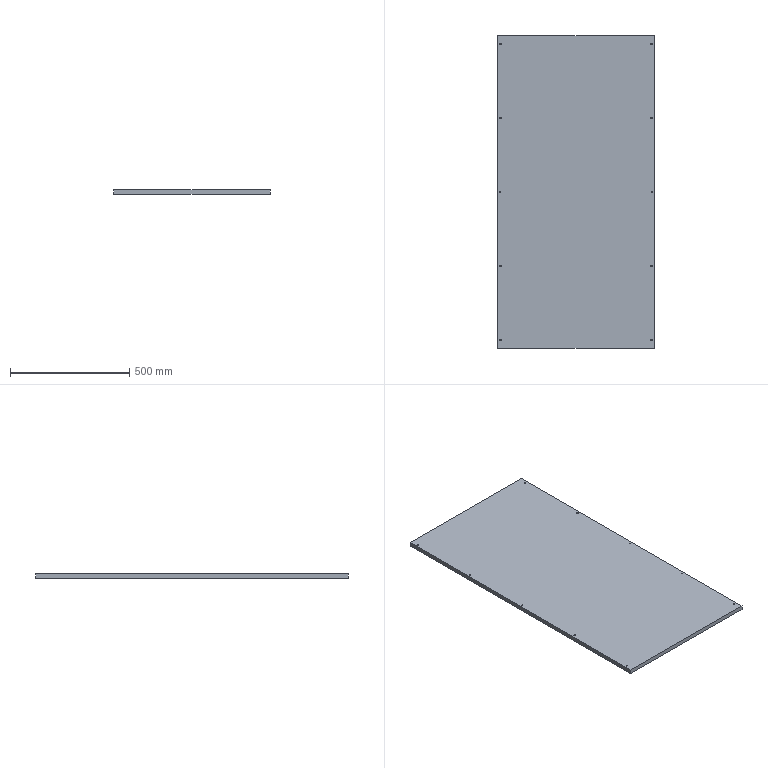Part | STEP file | DECAK NQ7A | 1 solid | 16 faces | box 658 x 1310 x 18 mm | volume 15510409 mm3 | cylinder 10 | plane 6 | commonest cylinder face diameters 6.5 x8 4 x2
STEP:
#1=CARTESIAN_POINT('',(0.,0.,0.));
#2=DIRECTION('',(0.,0.,1.));
#3=DIRECTION('',(1.,0.,0.));
#4=AXIS2_PLACEMENT_3D('',#1,#2,#3);
#5=CARTESIAN_POINT('',(320.75,-620.,9.));
#6=VERTEX_POINT('',#5);
#7=CARTESIAN_POINT('',(317.5,-620.,9.));
#8=DIRECTION('',(0.,0.,1.));
#9=DIRECTION('',(1.,0.,0.));
#10=AXIS2_PLACEMENT_3D('',#7,#8,#9);
#11=CIRCLE('',#10,3.25);
#12=CARTESIAN_POINT('',(329.,-655.,9.));
#13=DIRECTION('',(0.,0.,1.));
#14=DIRECTION('',(1.,0.,0.));
#15=AXIS2_PLACEMENT_3D('',#12,#13,#14);
#16=PLANE('',#15);
#17=CARTESIAN_POINT('',(-11.5,35.));
#18=DIRECTION('',(1.,0.));
#19=AXIS2_PLACEMENT_2D('',#17,#18);
#20=CIRCLE('',#19,3.25);
#21=(GEOMETRIC_REPRESENTATION_CONTEXT(2)PARAMETRIC_REPRESENTATION_CONTEXT()REPRESENTATION_CONTEXT('',''));
#22=DEFINITIONAL_REPRESENTATION('',(#20),#21);
#23=PCURVE('',#16,#22);
#24=CARTESIAN_POINT('',(317.5,-620.,9.));
#25=DIRECTION('',(0.,0.,-1.));
#26=DIRECTION('',(-1.,0.,0.));
#27=AXIS2_PLACEMENT_3D('',#24,#25,#26);
#28=CYLINDRICAL_SURFACE('',#27,3.25);
#29=CARTESIAN_POINT('',(9.425,0.));
#30=DIRECTION('',(-1.,0.));
#31=VECTOR('',#30,1.);
#32=LINE('',#29,#31);
#33=(GEOMETRIC_REPRESENTATION_CONTEXT(2)PARAMETRIC_REPRESENTATION_CONTEXT()REPRESENTATION_CONTEXT('',''));
#34=DEFINITIONAL_REPRESENTATION('',(#32),#33);
#35=PCURVE('',#28,#34);
#36=SURFACE_CURVE('',#11,(#23,#35),.PCURVE_S1.);
#37=EDGE_CURVE('',#6,#6,#36,.T.);
#38=ORIENTED_EDGE('',*,*,#37,.F.);
#39=EDGE_LOOP('',(#38));
#40=FACE_BOUND('',#39,.T.);
#41=CARTESIAN_POINT('',(320.75,-310.,9.));
#42=VERTEX_POINT('',#41);
#43=CARTESIAN_POINT('',(317.5,-310.,9.));
#44=DIRECTION('',(0.,0.,1.));
#45=DIRECTION('',(1.,0.,0.));
#46=AXIS2_PLACEMENT_3D('',#43,#44,#45);
#47=CIRCLE('',#46,3.25);
#48=CARTESIAN_POINT('',(-11.5,345.));
#49=DIRECTION('',(1.,0.));
#50=AXIS2_PLACEMENT_2D('',#48,#49);
#51=CIRCLE('',#50,3.25);
#52=(GEOMETRIC_REPRESENTATION_CONTEXT(2)PARAMETRIC_REPRESENTATION_CONTEXT()REPRESENTATION_CONTEXT('',''));
#53=DEFINITIONAL_REPRESENTATION('',(#51),#52);
#54=PCURVE('',#16,#53);
#55=CARTESIAN_POINT('',(317.5,-310.,9.));
#56=DIRECTION('',(0.,0.,-1.));
#57=DIRECTION('',(-1.,0.,0.));
#58=AXIS2_PLACEMENT_3D('',#55,#56,#57);
#59=CYLINDRICAL_SURFACE('',#58,3.25);
#60=CARTESIAN_POINT('',(9.425,0.));
#61=DIRECTION('',(-1.,0.));
#62=VECTOR('',#61,1.);
#63=LINE('',#60,#62);
#64=(GEOMETRIC_REPRESENTATION_CONTEXT(2)PARAMETRIC_REPRESENTATION_CONTEXT()REPRESENTATION_CONTEXT('',''));
#65=DEFINITIONAL_REPRESENTATION('',(#63),#64);
#66=PCURVE('',#59,#65);
#67=SURFACE_CURVE('',#47,(#54,#66),.PCURVE_S1.);
#68=EDGE_CURVE('',#42,#42,#67,.T.);
#69=ORIENTED_EDGE('',*,*,#68,.F.);
#70=EDGE_LOOP('',(#69));
#71=FACE_BOUND('',#70,.T.);
#72=CARTESIAN_POINT('',(319.5,0.,9.));
#73=VERTEX_POINT('',#72);
#74=CARTESIAN_POINT('',(317.5,0.,9.));
#75=DIRECTION('',(0.,0.,1.));
#76=DIRECTION('',(1.,0.,0.));
#77=AXIS2_PLACEMENT_3D('',#74,#75,#76);
#78=CIRCLE('',#77,2.);
#79=CARTESIAN_POINT('',(-11.5,655.));
#80=DIRECTION('',(1.,0.));
#81=AXIS2_PLACEMENT_2D('',#79,#80);
#82=CIRCLE('',#81,2.);
#83=(GEOMETRIC_REPRESENTATION_CONTEXT(2)PARAMETRIC_REPRESENTATION_CONTEXT()REPRESENTATION_CONTEXT('',''));
#84=DEFINITIONAL_REPRESENTATION('',(#82),#83);
#85=PCURVE('',#16,#84);
#86=CARTESIAN_POINT('',(317.5,0.,9.));
#87=DIRECTION('',(0.,0.,-1.));
#88=DIRECTION('',(-1.,0.,0.));
#89=AXIS2_PLACEMENT_3D('',#86,#87,#88);
#90=CYLINDRICAL_SURFACE('',#89,2.);
#91=CARTESIAN_POINT('',(9.425,0.));
#92=DIRECTION('',(-1.,0.));
#93=VECTOR('',#92,1.);
#94=LINE('',#91,#93);
#95=(GEOMETRIC_REPRESENTATION_CONTEXT(2)PARAMETRIC_REPRESENTATION_CONTEXT()REPRESENTATION_CONTEXT('',''));
#96=DEFINITIONAL_REPRESENTATION('',(#94),#95);
#97=PCURVE('',#90,#96);
#98=SURFACE_CURVE('',#78,(#85,#97),.PCURVE_S1.);
#99=EDGE_CURVE('',#73,#73,#98,.T.);
#100=ORIENTED_EDGE('',*,*,#99,.F.);
#101=EDGE_LOOP('',(#100));
#102=FACE_BOUND('',#101,.T.);
#103=CARTESIAN_POINT('',(-314.25,310.,9.));
#104=VERTEX_POINT('',#103);
#105=CARTESIAN_POINT('',(-317.5,310.,9.));
#106=DIRECTION('',(0.,0.,1.));
#107=DIRECTION('',(1.,0.,0.));
#108=AXIS2_PLACEMENT_3D('',#105,#106,#107);
#109=CIRCLE('',#108,3.25);
#110=CARTESIAN_POINT('',(-646.5,965.));
#111=DIRECTION('',(1.,0.));
#112=AXIS2_PLACEMENT_2D('',#110,#111);
#113=CIRCLE('',#112,3.25);
#114=(GEOMETRIC_REPRESENTATION_CONTEXT(2)PARAMETRIC_REPRESENTATION_CONTEXT()REPRESENTATION_CONTEXT('',''));
#115=DEFINITIONAL_REPRESENTATION('',(#113),#114);
#116=PCURVE('',#16,#115);
#117=CARTESIAN_POINT('',(-317.5,310.,9.));
#118=DIRECTION('',(0.,0.,-1.));
#119=DIRECTION('',(-1.,0.,0.));
#120=AXIS2_PLACEMENT_3D('',#117,#118,#119);
#121=CYLINDRICAL_SURFACE('',#120,3.25);
#122=CARTESIAN_POINT('',(9.425,0.));
#123=DIRECTION('',(-1.,0.));
#124=VECTOR('',#123,1.);
#125=LINE('',#122,#124);
#126=(GEOMETRIC_REPRESENTATION_CONTEXT(2)PARAMETRIC_REPRESENTATION_CONTEXT()REPRESENTATION_CONTEXT('',''));
#127=DEFINITIONAL_REPRESENTATION('',(#125),#126);
#128=PCURVE('',#121,#127);
#129=SURFACE_CURVE('',#109,(#116,#128),.PCURVE_S1.);
#130=EDGE_CURVE('',#104,#104,#129,.T.);
#131=ORIENTED_EDGE('',*,*,#130,.F.);
#132=EDGE_LOOP('',(#131));
#133=FACE_BOUND('',#132,.T.);
#134=CARTESIAN_POINT('',(320.75,620.,9.));
#135=VERTEX_POINT('',#134);
#136=CARTESIAN_POINT('',(317.5,620.,9.));
#137=DIRECTION('',(0.,0.,1.));
#138=DIRECTION('',(1.,0.,0.));
#139=AXIS2_PLACEMENT_3D('',#136,#137,#138);
#140=CIRCLE('',#139,3.25);
#141=CARTESIAN_POINT('',(-11.5,1275.));
#142=DIRECTION('',(1.,0.));
#143=AXIS2_PLACEMENT_2D('',#141,#142);
#144=CIRCLE('',#143,3.25);
#145=(GEOMETRIC_REPRESENTATION_CONTEXT(2)PARAMETRIC_REPRESENTATION_CONTEXT()REPRESENTATION_CONTEXT('',''));
#146=DEFINITIONAL_REPRESENTATION('',(#144),#145);
#147=PCURVE('',#16,#146);
#148=CARTESIAN_POINT('',(317.5,620.,9.));
#149=DIRECTION('',(0.,0.,-1.));
#150=DIRECTION('',(-1.,0.,0.));
#151=AXIS2_PLACEMENT_3D('',#148,#149,#150);
#152=CYLINDRICAL_SURFACE('',#151,3.25);
#153=CARTESIAN_POINT('',(9.425,0.));
#154=DIRECTION('',(-1.,0.));
#155=VECTOR('',#154,1.);
#156=LINE('',#153,#155);
#157=(GEOMETRIC_REPRESENTATION_CONTEXT(2)PARAMETRIC_REPRESENTATION_CONTEXT()REPRESENTATION_CONTEXT('',''));
#158=DEFINITIONAL_REPRESENTATION('',(#156),#157);
#159=PCURVE('',#152,#158);
#160=SURFACE_CURVE('',#140,(#147,#159),.PCURVE_S1.);
#161=EDGE_CURVE('',#135,#135,#160,.T.);
#162=ORIENTED_EDGE('',*,*,#161,.F.);
#163=EDGE_LOOP('',(#162));
#164=FACE_BOUND('',#163,.T.);
#165=CARTESIAN_POINT('',(329.,-655.,9.));
#166=VERTEX_POINT('',#165);
#167=CARTESIAN_POINT('',(329.,655.,9.));
#168=VERTEX_POINT('',#167);
#169=CARTESIAN_POINT('',(329.,655.,9.));
#170=DIRECTION('',(0.,1.,0.));
#171=VECTOR('',#170,1.);
#172=LINE('',#169,#171);
#173=CARTESIAN_POINT('',(0.,1310.));
#174=DIRECTION('',(0.,1.));
#175=VECTOR('',#174,1.);
#176=LINE('',#173,#175);
#177=(GEOMETRIC_REPRESENTATION_CONTEXT(2)PARAMETRIC_REPRESENTATION_CONTEXT()REPRESENTATION_CONTEXT('',''));
#178=DEFINITIONAL_REPRESENTATION('',(#176),#177);
#179=PCURVE('',#16,#178);
#180=CARTESIAN_POINT('',(329.,655.,9.));
#181=DIRECTION('',(-1.,0.,0.));
#182=DIRECTION('',(0.,0.,1.));
#183=AXIS2_PLACEMENT_3D('',#180,#181,#182);
#184=PLANE('',#183);
#185=CARTESIAN_POINT('',(0.,0.));
#186=DIRECTION('',(0.,1.));
#187=VECTOR('',#186,1.);
#188=LINE('',#185,#187);
#189=(GEOMETRIC_REPRESENTATION_CONTEXT(2)PARAMETRIC_REPRESENTATION_CONTEXT()REPRESENTATION_CONTEXT('',''));
#190=DEFINITIONAL_REPRESENTATION('',(#188),#189);
#191=PCURVE('',#184,#190);
#192=SURFACE_CURVE('',#172,(#179,#191),.PCURVE_S1.);
#193=EDGE_CURVE('',#166,#168,#192,.T.);
#194=ORIENTED_EDGE('',*,*,#193,.T.);
#195=CARTESIAN_POINT('',(-329.,655.,9.));
#196=VERTEX_POINT('',#195);
#197=CARTESIAN_POINT('',(-329.,655.,9.));
#198=DIRECTION('',(-1.,0.,0.));
#199=VECTOR('',#198,1.);
#200=LINE('',#197,#199);
#201=CARTESIAN_POINT('',(-658.,1310.));
#202=DIRECTION('',(-1.,0.));
#203=VECTOR('',#202,1.);
#204=LINE('',#201,#203);
#205=(GEOMETRIC_REPRESENTATION_CONTEXT(2)PARAMETRIC_REPRESENTATION_CONTEXT()REPRESENTATION_CONTEXT('',''));
#206=DEFINITIONAL_REPRESENTATION('',(#204),#205);
#207=PCURVE('',#16,#206);
#208=CARTESIAN_POINT('',(-329.,655.,9.));
#209=DIRECTION('',(0.,-1.,0.));
#210=DIRECTION('',(1.,0.,0.));
#211=AXIS2_PLACEMENT_3D('',#208,#209,#210);
#212=PLANE('',#211);
#213=CARTESIAN_POINT('',(0.,0.));
#214=DIRECTION('',(-1.,0.));
#215=VECTOR('',#214,1.);
#216=LINE('',#213,#215);
#217=(GEOMETRIC_REPRESENTATION_CONTEXT(2)PARAMETRIC_REPRESENTATION_CONTEXT()REPRESENTATION_CONTEXT('',''));
#218=DEFINITIONAL_REPRESENTATION('',(#216),#217);
#219=PCURVE('',#212,#218);
#220=SURFACE_CURVE('',#200,(#207,#219),.PCURVE_S1.);
#221=EDGE_CURVE('',#168,#196,#220,.T.);
#222=ORIENTED_EDGE('',*,*,#221,.T.);
#223=CARTESIAN_POINT('',(-329.,-655.,9.));
#224=VERTEX_POINT('',#223);
#225=CARTESIAN_POINT('',(-329.,655.,9.));
#226=DIRECTION('',(0.,-1.,0.));
#227=VECTOR('',#226,1.);
#228=LINE('',#225,#227);
#229=CARTESIAN_POINT('',(-658.,1310.));
#230=DIRECTION('',(0.,-1.));
#231=VECTOR('',#230,1.);
#232=LINE('',#229,#231);
#233=(GEOMETRIC_REPRESENTATION_CONTEXT(2)PARAMETRIC_REPRESENTATION_CONTEXT()REPRESENTATION_CONTEXT('',''));
#234=DEFINITIONAL_REPRESENTATION('',(#232),#233);
#235=PCURVE('',#16,#234);
#236=CARTESIAN_POINT('',(-329.,655.,9.));
#237=DIRECTION('',(1.,0.,0.));
#238=DIRECTION('',(0.,0.,-1.));
#239=AXIS2_PLACEMENT_3D('',#236,#237,#238);
#240=PLANE('',#239);
#241=CARTESIAN_POINT('',(0.,0.));
#242=DIRECTION('',(0.,-1.));
#243=VECTOR('',#242,1.);
#244=LINE('',#241,#243);
#245=(GEOMETRIC_REPRESENTATION_CONTEXT(2)PARAMETRIC_REPRESENTATION_CONTEXT()REPRESENTATION_CONTEXT('',''));
#246=DEFINITIONAL_REPRESENTATION('',(#244),#245);
#247=PCURVE('',#240,#246);
#248=SURFACE_CURVE('',#228,(#235,#247),.PCURVE_S1.);
#249=EDGE_CURVE('',#196,#224,#248,.T.);
#250=ORIENTED_EDGE('',*,*,#249,.T.);
#251=CARTESIAN_POINT('',(-329.,-655.,9.));
#252=DIRECTION('',(1.,0.,0.));
#253=VECTOR('',#252,1.);
#254=LINE('',#251,#253);
#255=CARTESIAN_POINT('',(-658.,0.));
#256=DIRECTION('',(1.,0.));
#257=VECTOR('',#256,1.);
#258=LINE('',#255,#257);
#259=(GEOMETRIC_REPRESENTATION_CONTEXT(2)PARAMETRIC_REPRESENTATION_CONTEXT()REPRESENTATION_CONTEXT('',''));
#260=DEFINITIONAL_REPRESENTATION('',(#258),#259);
#261=PCURVE('',#16,#260);
#262=CARTESIAN_POINT('',(-329.,-655.,9.));
#263=DIRECTION('',(0.,1.,0.));
#264=DIRECTION('',(-1.,0.,0.));
#265=AXIS2_PLACEMENT_3D('',#262,#263,#264);
#266=PLANE('',#265);
#267=CARTESIAN_POINT('',(0.,0.));
#268=DIRECTION('',(-1.,0.));
#269=VECTOR('',#268,1.);
#270=LINE('',#267,#269);
#271=(GEOMETRIC_REPRESENTATION_CONTEXT(2)PARAMETRIC_REPRESENTATION_CONTEXT()REPRESENTATION_CONTEXT('',''));
#272=DEFINITIONAL_REPRESENTATION('',(#270),#271);
#273=PCURVE('',#266,#272);
#274=SURFACE_CURVE('',#254,(#261,#273),.PCURVE_S1.);
#275=EDGE_CURVE('',#224,#166,#274,.T.);
#276=ORIENTED_EDGE('',*,*,#275,.T.);
#277=EDGE_LOOP('',(#194,#222,#250,#276));
#278=FACE_BOUND('',#277,.T.);
#279=CARTESIAN_POINT('',(-314.25,620.,9.));
#280=VERTEX_POINT('',#279);
#281=CARTESIAN_POINT('',(-317.5,620.,9.));
#282=DIRECTION('',(0.,0.,1.));
#283=DIRECTION('',(1.,0.,0.));
#284=AXIS2_PLACEMENT_3D('',#281,#282,#283);
#285=CIRCLE('',#284,3.25);
#286=CARTESIAN_POINT('',(-646.5,1275.));
#287=DIRECTION('',(1.,0.));
#288=AXIS2_PLACEMENT_2D('',#286,#287);
#289=CIRCLE('',#288,3.25);
#290=(GEOMETRIC_REPRESENTATION_CONTEXT(2)PARAMETRIC_REPRESENTATION_CONTEXT()REPRESENTATION_CONTEXT('',''));
#291=DEFINITIONAL_REPRESENTATION('',(#289),#290);
#292=PCURVE('',#16,#291);
#293=CARTESIAN_POINT('',(-317.5,620.,9.));
#294=DIRECTION('',(0.,0.,-1.));
#295=DIRECTION('',(-1.,0.,0.));
#296=AXIS2_PLACEMENT_3D('',#293,#294,#295);
#297=CYLINDRICAL_SURFACE('',#296,3.25);
#298=CARTESIAN_POINT('',(9.425,0.));
#299=DIRECTION('',(-1.,0.));
#300=VECTOR('',#299,1.);
#301=LINE('',#298,#300);
#302=(GEOMETRIC_REPRESENTATION_CONTEXT(2)PARAMETRIC_REPRESENTATION_CONTEXT()REPRESENTATION_CONTEXT('',''));
#303=DEFINITIONAL_REPRESENTATION('',(#301),#302);
#304=PCURVE('',#297,#303);
#305=SURFACE_CURVE('',#285,(#292,#304),.PCURVE_S1.);
#306=EDGE_CURVE('',#280,#280,#305,.T.);
#307=ORIENTED_EDGE('',*,*,#306,.F.);
#308=EDGE_LOOP('',(#307));
#309=FACE_BOUND('',#308,.T.);
#310=CARTESIAN_POINT('',(320.75,310.,9.));
#311=VERTEX_POINT('',#310);
#312=CARTESIAN_POINT('',(317.5,310.,9.));
#313=DIRECTION('',(0.,0.,1.));
#314=DIRECTION('',(1.,0.,0.));
#315=AXIS2_PLACEMENT_3D('',#312,#313,#314);
#316=CIRCLE('',#315,3.25);
#317=CARTESIAN_POINT('',(-11.5,965.));
#318=DIRECTION('',(1.,0.));
#319=AXIS2_PLACEMENT_2D('',#317,#318);
#320=CIRCLE('',#319,3.25);
#321=(GEOMETRIC_REPRESENTATION_CONTEXT(2)PARAMETRIC_REPRESENTATION_CONTEXT()REPRESENTATION_CONTEXT('',''));
#322=DEFINITIONAL_REPRESENTATION('',(#320),#321);
#323=PCURVE('',#16,#322);
#324=CARTESIAN_POINT('',(317.5,310.,9.));
#325=DIRECTION('',(0.,0.,-1.));
#326=DIRECTION('',(-1.,0.,0.));
#327=AXIS2_PLACEMENT_3D('',#324,#325,#326);
#328=CYLINDRICAL_SURFACE('',#327,3.25);
#329=CARTESIAN_POINT('',(9.425,0.));
#330=DIRECTION('',(-1.,0.));
#331=VECTOR('',#330,1.);
#332=LINE('',#329,#331);
#333=(GEOMETRIC_REPRESENTATION_CONTEXT(2)PARAMETRIC_REPRESENTATION_CONTEXT()REPRESENTATION_CONTEXT('',''));
#334=DEFINITIONAL_REPRESENTATION('',(#332),#333);
#335=PCURVE('',#328,#334);
#336=SURFACE_CURVE('',#316,(#323,#335),.PCURVE_S1.);
#337=EDGE_CURVE('',#311,#311,#336,.T.);
#338=ORIENTED_EDGE('',*,*,#337,.F.);
#339=EDGE_LOOP('',(#338));
#340=FACE_BOUND('',#339,.T.);
#341=CARTESIAN_POINT('',(-314.25,-310.,9.));
#342=VERTEX_POINT('',#341);
#343=CARTESIAN_POINT('',(-317.5,-310.,9.));
#344=DIRECTION('',(0.,0.,1.));
#345=DIRECTION('',(1.,0.,0.));
#346=AXIS2_PLACEMENT_3D('',#343,#344,#345);
#347=CIRCLE('',#346,3.25);
#348=CARTESIAN_POINT('',(-646.5,345.));
#349=DIRECTION('',(1.,0.));
#350=AXIS2_PLACEMENT_2D('',#348,#349);
#351=CIRCLE('',#350,3.25);
#352=(GEOMETRIC_REPRESENTATION_CONTEXT(2)PARAMETRIC_REPRESENTATION_CONTEXT()REPRESENTATION_CONTEXT('',''));
#353=DEFINITIONAL_REPRESENTATION('',(#351),#352);
#354=PCURVE('',#16,#353);
#355=CARTESIAN_POINT('',(-317.5,-310.,9.));
#356=DIRECTION('',(0.,0.,-1.));
#357=DIRECTION('',(-1.,0.,0.));
#358=AXIS2_PLACEMENT_3D('',#355,#356,#357);
#359=CYLINDRICAL_SURFACE('',#358,3.25);
#360=CARTESIAN_POINT('',(9.425,0.));
#361=DIRECTION('',(-1.,0.));
#362=VECTOR('',#361,1.);
#363=LINE('',#360,#362);
#364=(GEOMETRIC_REPRESENTATION_CONTEXT(2)PARAMETRIC_REPRESENTATION_CONTEXT()REPRESENTATION_CONTEXT('',''));
#365=DEFINITIONAL_REPRESENTATION('',(#363),#364);
#366=PCURVE('',#359,#365);
#367=SURFACE_CURVE('',#347,(#354,#366),.PCURVE_S1.);
#368=EDGE_CURVE('',#342,#342,#367,.T.);
#369=ORIENTED_EDGE('',*,*,#368,.F.);
#370=EDGE_LOOP('',(#369));
#371=FACE_BOUND('',#370,.T.);
#372=CARTESIAN_POINT('',(-314.25,-620.,9.));
#373=VERTEX_POINT('',#372);
#374=CARTESIAN_POINT('',(-317.5,-620.,9.));
#375=DIRECTION('',(0.,0.,1.));
#376=DIRECTION('',(1.,0.,0.));
#377=AXIS2_PLACEMENT_3D('',#374,#375,#376);
#378=CIRCLE('',#377,3.25);
#379=CARTESIAN_POINT('',(-646.5,35.));
#380=DIRECTION('',(1.,0.));
#381=AXIS2_PLACEMENT_2D('',#379,#380);
#382=CIRCLE('',#381,3.25);
#383=(GEOMETRIC_REPRESENTATION_CONTEXT(2)PARAMETRIC_REPRESENTATION_CONTEXT()REPRESENTATION_CONTEXT('',''));
#384=DEFINITIONAL_REPRESENTATION('',(#382),#383);
#385=PCURVE('',#16,#384);
#386=CARTESIAN_POINT('',(-317.5,-620.,9.));
#387=DIRECTION('',(0.,0.,-1.));
#388=DIRECTION('',(-1.,0.,0.));
#389=AXIS2_PLACEMENT_3D('',#386,#387,#388);
#390=CYLINDRICAL_SURFACE('',#389,3.25);
#391=CARTESIAN_POINT('',(9.425,0.));
#392=DIRECTION('',(-1.,0.));
#393=VECTOR('',#392,1.);
#394=LINE('',#391,#393);
#395=(GEOMETRIC_REPRESENTATION_CONTEXT(2)PARAMETRIC_REPRESENTATION_CONTEXT()REPRESENTATION_CONTEXT('',''));
#396=DEFINITIONAL_REPRESENTATION('',(#394),#395);
#397=PCURVE('',#390,#396);
#398=SURFACE_CURVE('',#378,(#385,#397),.PCURVE_S1.);
#399=EDGE_CURVE('',#373,#373,#398,.T.);
#400=ORIENTED_EDGE('',*,*,#399,.F.);
#401=EDGE_LOOP('',(#400));
#402=FACE_BOUND('',#401,.T.);
#403=CARTESIAN_POINT('',(-315.5,0.,9.));
#404=VERTEX_POINT('',#403);
#405=CARTESIAN_POINT('',(-317.5,0.,9.));
#406=DIRECTION('',(0.,0.,1.));
#407=DIRECTION('',(1.,0.,0.));
#408=AXIS2_PLACEMENT_3D('',#405,#406,#407);
#409=CIRCLE('',#408,2.);
#410=CARTESIAN_POINT('',(-646.5,655.));
#411=DIRECTION('',(1.,0.));
#412=AXIS2_PLACEMENT_2D('',#410,#411);
#413=CIRCLE('',#412,2.);
#414=(GEOMETRIC_REPRESENTATION_CONTEXT(2)PARAMETRIC_REPRESENTATION_CONTEXT()REPRESENTATION_CONTEXT('',''));
#415=DEFINITIONAL_REPRESENTATION('',(#413),#414);
#416=PCURVE('',#16,#415);
#417=CARTESIAN_POINT('',(-317.5,0.,9.));
#418=DIRECTION('',(0.,0.,-1.));
#419=DIRECTION('',(-1.,0.,0.));
#420=AXIS2_PLACEMENT_3D('',#417,#418,#419);
#421=CYLINDRICAL_SURFACE('',#420,2.);
#422=CARTESIAN_POINT('',(9.425,0.));
#423=DIRECTION('',(-1.,0.));
#424=VECTOR('',#423,1.);
#425=LINE('',#422,#424);
#426=(GEOMETRIC_REPRESENTATION_CONTEXT(2)PARAMETRIC_REPRESENTATION_CONTEXT()REPRESENTATION_CONTEXT('',''));
#427=DEFINITIONAL_REPRESENTATION('',(#425),#426);
#428=PCURVE('',#421,#427);
#429=SURFACE_CURVE('',#409,(#416,#428),.PCURVE_S1.);
#430=EDGE_CURVE('',#404,#404,#429,.T.);
#431=ORIENTED_EDGE('',*,*,#430,.F.);
#432=EDGE_LOOP('',(#431));
#433=FACE_BOUND('',#432,.T.);
#434=ADVANCED_FACE('',(#40,#71,#102,#133,#164,#278,#309,#340,#371,#402,#433),#16,.T.);
#435=CARTESIAN_POINT('',(320.75,-620.,-9.));
#436=VERTEX_POINT('',#435);
#437=CARTESIAN_POINT('',(317.5,-620.,-9.));
#438=DIRECTION('',(0.,0.,1.));
#439=DIRECTION('',(1.,0.,0.));
#440=AXIS2_PLACEMENT_3D('',#437,#438,#439);
#441=CIRCLE('',#440,3.25);
#442=CARTESIAN_POINT('',(329.,-655.,-9.));
#443=DIRECTION('',(0.,0.,1.));
#444=DIRECTION('',(1.,0.,0.));
#445=AXIS2_PLACEMENT_3D('',#442,#443,#444);
#446=PLANE('',#445);
#447=CARTESIAN_POINT('',(-11.5,35.));
#448=DIRECTION('',(1.,0.));
#449=AXIS2_PLACEMENT_2D('',#447,#448);
#450=CIRCLE('',#449,3.25);
#451=(GEOMETRIC_REPRESENTATION_CONTEXT(2)PARAMETRIC_REPRESENTATION_CONTEXT()REPRESENTATION_CONTEXT('',''));
#452=DEFINITIONAL_REPRESENTATION('',(#450),#451);
#453=PCURVE('',#446,#452);
#454=CARTESIAN_POINT('',(9.425,18.));
#455=DIRECTION('',(-1.,0.));
#456=VECTOR('',#455,1.);
#457=LINE('',#454,#456);
#458=(GEOMETRIC_REPRESENTATION_CONTEXT(2)PARAMETRIC_REPRESENTATION_CONTEXT()REPRESENTATION_CONTEXT('',''));
#459=DEFINITIONAL_REPRESENTATION('',(#457),#458);
#460=PCURVE('',#28,#459);
#461=SURFACE_CURVE('',#441,(#453,#460),.PCURVE_S1.);
#462=EDGE_CURVE('',#436,#436,#461,.T.);
#463=ORIENTED_EDGE('',*,*,#462,.T.);
#464=EDGE_LOOP('',(#463));
#465=FACE_BOUND('',#464,.T.);
#466=CARTESIAN_POINT('',(320.75,-310.,-9.));
#467=VERTEX_POINT('',#466);
#468=CARTESIAN_POINT('',(317.5,-310.,-9.));
#469=DIRECTION('',(0.,0.,1.));
#470=DIRECTION('',(1.,0.,0.));
#471=AXIS2_PLACEMENT_3D('',#468,#469,#470);
#472=CIRCLE('',#471,3.25);
#473=CARTESIAN_POINT('',(-11.5,345.));
#474=DIRECTION('',(1.,0.));
#475=AXIS2_PLACEMENT_2D('',#473,#474);
#476=CIRCLE('',#475,3.25);
#477=(GEOMETRIC_REPRESENTATION_CONTEXT(2)PARAMETRIC_REPRESENTATION_CONTEXT()REPRESENTATION_CONTEXT('',''));
#478=DEFINITIONAL_REPRESENTATION('',(#476),#477);
#479=PCURVE('',#446,#478);
#480=CARTESIAN_POINT('',(9.425,18.));
#481=DIRECTION('',(-1.,0.));
#482=VECTOR('',#481,1.);
#483=LINE('',#480,#482);
#484=(GEOMETRIC_REPRESENTATION_CONTEXT(2)PARAMETRIC_REPRESENTATION_CONTEXT()REPRESENTATION_CONTEXT('',''));
#485=DEFINITIONAL_REPRESENTATION('',(#483),#484);
#486=PCURVE('',#59,#485);
#487=SURFACE_CURVE('',#472,(#479,#486),.PCURVE_S1.);
#488=EDGE_CURVE('',#467,#467,#487,.T.);
#489=ORIENTED_EDGE('',*,*,#488,.T.);
#490=EDGE_LOOP('',(#489));
#491=FACE_BOUND('',#490,.T.);
#492=CARTESIAN_POINT('',(319.5,0.,-9.));
#493=VERTEX_POINT('',#492);
#494=CARTESIAN_POINT('',(317.5,0.,-9.));
#495=DIRECTION('',(0.,0.,1.));
#496=DIRECTION('',(1.,0.,0.));
#497=AXIS2_PLACEMENT_3D('',#494,#495,#496);
#498=CIRCLE('',#497,2.);
#499=CARTESIAN_POINT('',(-11.5,655.));
#500=DIRECTION('',(1.,0.));
#501=AXIS2_PLACEMENT_2D('',#499,#500);
#502=CIRCLE('',#501,2.);
#503=(GEOMETRIC_REPRESENTATION_CONTEXT(2)PARAMETRIC_REPRESENTATION_CONTEXT()REPRESENTATION_CONTEXT('',''));
#504=DEFINITIONAL_REPRESENTATION('',(#502),#503);
#505=PCURVE('',#446,#504);
#506=CARTESIAN_POINT('',(9.425,18.));
#507=DIRECTION('',(-1.,0.));
#508=VECTOR('',#507,1.);
#509=LINE('',#506,#508);
#510=(GEOMETRIC_REPRESENTATION_CONTEXT(2)PARAMETRIC_REPRESENTATION_CONTEXT()REPRESENTATION_CONTEXT('',''));
#511=DEFINITIONAL_REPRESENTATION('',(#509),#510);
#512=PCURVE('',#90,#511);
#513=SURFACE_CURVE('',#498,(#505,#512),.PCURVE_S1.);
#514=EDGE_CURVE('',#493,#493,#513,.T.);
#515=ORIENTED_EDGE('',*,*,#514,.T.);
#516=EDGE_LOOP('',(#515));
#517=FACE_BOUND('',#516,.T.);
#518=CARTESIAN_POINT('',(-314.25,310.,-9.));
#519=VERTEX_POINT('',#518);
#520=CARTESIAN_POINT('',(-317.5,310.,-9.));
#521=DIRECTION('',(0.,0.,1.));
#522=DIRECTION('',(1.,0.,0.));
#523=AXIS2_PLACEMENT_3D('',#520,#521,#522);
#524=CIRCLE('',#523,3.25);
#525=CARTESIAN_POINT('',(-646.5,965.));
#526=DIRECTION('',(1.,0.));
#527=AXIS2_PLACEMENT_2D('',#525,#526);
#528=CIRCLE('',#527,3.25);
#529=(GEOMETRIC_REPRESENTATION_CONTEXT(2)PARAMETRIC_REPRESENTATION_CONTEXT()REPRESENTATION_CONTEXT('',''));
#530=DEFINITIONAL_REPRESENTATION('',(#528),#529);
#531=PCURVE('',#446,#530);
#532=CARTESIAN_POINT('',(9.425,18.));
#533=DIRECTION('',(-1.,0.));
#534=VECTOR('',#533,1.);
#535=LINE('',#532,#534);
#536=(GEOMETRIC_REPRESENTATION_CONTEXT(2)PARAMETRIC_REPRESENTATION_CONTEXT()REPRESENTATION_CONTEXT('',''));
#537=DEFINITIONAL_REPRESENTATION('',(#535),#536);
#538=PCURVE('',#121,#537);
#539=SURFACE_CURVE('',#524,(#531,#538),.PCURVE_S1.);
#540=EDGE_CURVE('',#519,#519,#539,.T.);
#541=ORIENTED_EDGE('',*,*,#540,.T.);
#542=EDGE_LOOP('',(#541));
#543=FACE_BOUND('',#542,.T.);
#544=CARTESIAN_POINT('',(320.75,620.,-9.));
#545=VERTEX_POINT('',#544);
#546=CARTESIAN_POINT('',(317.5,620.,-9.));
#547=DIRECTION('',(0.,0.,1.));
#548=DIRECTION('',(1.,0.,0.));
#549=AXIS2_PLACEMENT_3D('',#546,#547,#548);
#550=CIRCLE('',#549,3.25);
#551=CARTESIAN_POINT('',(-11.5,1275.));
#552=DIRECTION('',(1.,0.));
#553=AXIS2_PLACEMENT_2D('',#551,#552);
#554=CIRCLE('',#553,3.25);
#555=(GEOMETRIC_REPRESENTATION_CONTEXT(2)PARAMETRIC_REPRESENTATION_CONTEXT()REPRESENTATION_CONTEXT('',''));
#556=DEFINITIONAL_REPRESENTATION('',(#554),#555);
#557=PCURVE('',#446,#556);
#558=CARTESIAN_POINT('',(9.425,18.));
#559=DIRECTION('',(-1.,0.));
#560=VECTOR('',#559,1.);
#561=LINE('',#558,#560);
#562=(GEOMETRIC_REPRESENTATION_CONTEXT(2)PARAMETRIC_REPRESENTATION_CONTEXT()REPRESENTATION_CONTEXT('',''));
#563=DEFINITIONAL_REPRESENTATION('',(#561),#562);
#564=PCURVE('',#152,#563);
#565=SURFACE_CURVE('',#550,(#557,#564),.PCURVE_S1.);
#566=EDGE_CURVE('',#545,#545,#565,.T.);
#567=ORIENTED_EDGE('',*,*,#566,.T.);
#568=EDGE_LOOP('',(#567));
#569=FACE_BOUND('',#568,.T.);
#570=CARTESIAN_POINT('',(329.,-655.,-9.));
#571=VERTEX_POINT('',#570);
#572=CARTESIAN_POINT('',(329.,655.,-9.));
#573=VERTEX_POINT('',#572);
#574=CARTESIAN_POINT('',(329.,655.,-9.));
#575=DIRECTION('',(0.,1.,0.));
#576=VECTOR('',#575,1.);
#577=LINE('',#574,#576);
#578=CARTESIAN_POINT('',(0.,1310.));
#579=DIRECTION('',(0.,1.));
#580=VECTOR('',#579,1.);
#581=LINE('',#578,#580);
#582=(GEOMETRIC_REPRESENTATION_CONTEXT(2)PARAMETRIC_REPRESENTATION_CONTEXT()REPRESENTATION_CONTEXT('',''));
#583=DEFINITIONAL_REPRESENTATION('',(#581),#582);
#584=PCURVE('',#446,#583);
#585=CARTESIAN_POINT('',(-18.,0.));
#586=DIRECTION('',(0.,1.));
#587=VECTOR('',#586,1.);
#588=LINE('',#585,#587);
#589=(GEOMETRIC_REPRESENTATION_CONTEXT(2)PARAMETRIC_REPRESENTATION_CONTEXT()REPRESENTATION_CONTEXT('',''));
#590=DEFINITIONAL_REPRESENTATION('',(#588),#589);
#591=PCURVE('',#184,#590);
#592=SURFACE_CURVE('',#577,(#584,#591),.PCURVE_S1.);
#593=EDGE_CURVE('',#571,#573,#592,.T.);
#594=ORIENTED_EDGE('',*,*,#593,.F.);
#595=CARTESIAN_POINT('',(-329.,-655.,-9.));
#596=VERTEX_POINT('',#595);
#597=CARTESIAN_POINT('',(-329.,-655.,-9.));
#598=DIRECTION('',(1.,0.,0.));
#599=VECTOR('',#598,1.);
#600=LINE('',#597,#599);
#601=CARTESIAN_POINT('',(-658.,0.));
#602=DIRECTION('',(1.,0.));
#603=VECTOR('',#602,1.);
#604=LINE('',#601,#603);
#605=(GEOMETRIC_REPRESENTATION_CONTEXT(2)PARAMETRIC_REPRESENTATION_CONTEXT()REPRESENTATION_CONTEXT('',''));
#606=DEFINITIONAL_REPRESENTATION('',(#604),#605);
#607=PCURVE('',#446,#606);
#608=CARTESIAN_POINT('',(0.,-18.));
#609=DIRECTION('',(-1.,0.));
#610=VECTOR('',#609,1.);
#611=LINE('',#608,#610);
#612=(GEOMETRIC_REPRESENTATION_CONTEXT(2)PARAMETRIC_REPRESENTATION_CONTEXT()REPRESENTATION_CONTEXT('',''));
#613=DEFINITIONAL_REPRESENTATION('',(#611),#612);
#614=PCURVE('',#266,#613);
#615=SURFACE_CURVE('',#600,(#607,#614),.PCURVE_S1.);
#616=EDGE_CURVE('',#596,#571,#615,.T.);
#617=ORIENTED_EDGE('',*,*,#616,.F.);
#618=CARTESIAN_POINT('',(-329.,655.,-9.));
#619=VERTEX_POINT('',#618);
#620=CARTESIAN_POINT('',(-329.,655.,-9.));
#621=DIRECTION('',(0.,-1.,0.));
#622=VECTOR('',#621,1.);
#623=LINE('',#620,#622);
#624=CARTESIAN_POINT('',(-658.,1310.));
#625=DIRECTION('',(0.,-1.));
#626=VECTOR('',#625,1.);
#627=LINE('',#624,#626);
#628=(GEOMETRIC_REPRESENTATION_CONTEXT(2)PARAMETRIC_REPRESENTATION_CONTEXT()REPRESENTATION_CONTEXT('',''));
#629=DEFINITIONAL_REPRESENTATION('',(#627),#628);
#630=PCURVE('',#446,#629);
#631=CARTESIAN_POINT('',(18.,0.));
#632=DIRECTION('',(0.,-1.));
#633=VECTOR('',#632,1.);
#634=LINE('',#631,#633);
#635=(GEOMETRIC_REPRESENTATION_CONTEXT(2)PARAMETRIC_REPRESENTATION_CONTEXT()REPRESENTATION_CONTEXT('',''));
#636=DEFINITIONAL_REPRESENTATION('',(#634),#635);
#637=PCURVE('',#240,#636);
#638=SURFACE_CURVE('',#623,(#630,#637),.PCURVE_S1.);
#639=EDGE_CURVE('',#619,#596,#638,.T.);
#640=ORIENTED_EDGE('',*,*,#639,.F.);
#641=CARTESIAN_POINT('',(-329.,655.,-9.));
#642=DIRECTION('',(-1.,0.,0.));
#643=VECTOR('',#642,1.);
#644=LINE('',#641,#643);
#645=CARTESIAN_POINT('',(-658.,1310.));
#646=DIRECTION('',(-1.,0.));
#647=VECTOR('',#646,1.);
#648=LINE('',#645,#647);
#649=(GEOMETRIC_REPRESENTATION_CONTEXT(2)PARAMETRIC_REPRESENTATION_CONTEXT()REPRESENTATION_CONTEXT('',''));
#650=DEFINITIONAL_REPRESENTATION('',(#648),#649);
#651=PCURVE('',#446,#650);
#652=CARTESIAN_POINT('',(0.,-18.));
#653=DIRECTION('',(-1.,0.));
#654=VECTOR('',#653,1.);
#655=LINE('',#652,#654);
#656=(GEOMETRIC_REPRESENTATION_CONTEXT(2)PARAMETRIC_REPRESENTATION_CONTEXT()REPRESENTATION_CONTEXT('',''));
#657=DEFINITIONAL_REPRESENTATION('',(#655),#656);
#658=PCURVE('',#212,#657);
#659=SURFACE_CURVE('',#644,(#651,#658),.PCURVE_S1.);
#660=EDGE_CURVE('',#573,#619,#659,.T.);
#661=ORIENTED_EDGE('',*,*,#660,.F.);
#662=EDGE_LOOP('',(#594,#617,#640,#661));
#663=FACE_BOUND('',#662,.T.);
#664=CARTESIAN_POINT('',(-314.25,620.,-9.));
#665=VERTEX_POINT('',#664);
#666=CARTESIAN_POINT('',(-317.5,620.,-9.));
#667=DIRECTION('',(0.,0.,1.));
#668=DIRECTION('',(1.,0.,0.));
#669=AXIS2_PLACEMENT_3D('',#666,#667,#668);
#670=CIRCLE('',#669,3.25);
#671=CARTESIAN_POINT('',(-646.5,1275.));
#672=DIRECTION('',(1.,0.));
#673=AXIS2_PLACEMENT_2D('',#671,#672);
#674=CIRCLE('',#673,3.25);
#675=(GEOMETRIC_REPRESENTATION_CONTEXT(2)PARAMETRIC_REPRESENTATION_CONTEXT()REPRESENTATION_CONTEXT('',''));
#676=DEFINITIONAL_REPRESENTATION('',(#674),#675);
#677=PCURVE('',#446,#676);
#678=CARTESIAN_POINT('',(9.425,18.));
#679=DIRECTION('',(-1.,0.));
#680=VECTOR('',#679,1.);
#681=LINE('',#678,#680);
#682=(GEOMETRIC_REPRESENTATION_CONTEXT(2)PARAMETRIC_REPRESENTATION_CONTEXT()REPRESENTATION_CONTEXT('',''));
#683=DEFINITIONAL_REPRESENTATION('',(#681),#682);
#684=PCURVE('',#297,#683);
#685=SURFACE_CURVE('',#670,(#677,#684),.PCURVE_S1.);
#686=EDGE_CURVE('',#665,#665,#685,.T.);
#687=ORIENTED_EDGE('',*,*,#686,.T.);
#688=EDGE_LOOP('',(#687));
#689=FACE_BOUND('',#688,.T.);
#690=CARTESIAN_POINT('',(320.75,310.,-9.));
#691=VERTEX_POINT('',#690);
#692=CARTESIAN_POINT('',(317.5,310.,-9.));
#693=DIRECTION('',(0.,0.,1.));
#694=DIRECTION('',(1.,0.,0.));
#695=AXIS2_PLACEMENT_3D('',#692,#693,#694);
#696=CIRCLE('',#695,3.25);
#697=CARTESIAN_POINT('',(-11.5,965.));
#698=DIRECTION('',(1.,0.));
#699=AXIS2_PLACEMENT_2D('',#697,#698);
#700=CIRCLE('',#699,3.25);
#701=(GEOMETRIC_REPRESENTATION_CONTEXT(2)PARAMETRIC_REPRESENTATION_CONTEXT()REPRESENTATION_CONTEXT('',''));
#702=DEFINITIONAL_REPRESENTATION('',(#700),#701);
#703=PCURVE('',#446,#702);
#704=CARTESIAN_POINT('',(9.425,18.));
#705=DIRECTION('',(-1.,0.));
#706=VECTOR('',#705,1.);
#707=LINE('',#704,#706);
#708=(GEOMETRIC_REPRESENTATION_CONTEXT(2)PARAMETRIC_REPRESENTATION_CONTEXT()REPRESENTATION_CONTEXT('',''));
#709=DEFINITIONAL_REPRESENTATION('',(#707),#708);
#710=PCURVE('',#328,#709);
#711=SURFACE_CURVE('',#696,(#703,#710),.PCURVE_S1.);
#712=EDGE_CURVE('',#691,#691,#711,.T.);
#713=ORIENTED_EDGE('',*,*,#712,.T.);
#714=EDGE_LOOP('',(#713));
#715=FACE_BOUND('',#714,.T.);
#716=CARTESIAN_POINT('',(-314.25,-310.,-9.));
#717=VERTEX_POINT('',#716);
#718=CARTESIAN_POINT('',(-317.5,-310.,-9.));
#719=DIRECTION('',(0.,0.,1.));
#720=DIRECTION('',(1.,0.,0.));
#721=AXIS2_PLACEMENT_3D('',#718,#719,#720);
#722=CIRCLE('',#721,3.25);
#723=CARTESIAN_POINT('',(-646.5,345.));
#724=DIRECTION('',(1.,0.));
#725=AXIS2_PLACEMENT_2D('',#723,#724);
#726=CIRCLE('',#725,3.25);
#727=(GEOMETRIC_REPRESENTATION_CONTEXT(2)PARAMETRIC_REPRESENTATION_CONTEXT()REPRESENTATION_CONTEXT('',''));
#728=DEFINITIONAL_REPRESENTATION('',(#726),#727);
#729=PCURVE('',#446,#728);
#730=CARTESIAN_POINT('',(9.425,18.));
#731=DIRECTION('',(-1.,0.));
#732=VECTOR('',#731,1.);
#733=LINE('',#730,#732);
#734=(GEOMETRIC_REPRESENTATION_CONTEXT(2)PARAMETRIC_REPRESENTATION_CONTEXT()REPRESENTATION_CONTEXT('',''));
#735=DEFINITIONAL_REPRESENTATION('',(#733),#734);
#736=PCURVE('',#359,#735);
#737=SURFACE_CURVE('',#722,(#729,#736),.PCURVE_S1.);
#738=EDGE_CURVE('',#717,#717,#737,.T.);
#739=ORIENTED_EDGE('',*,*,#738,.T.);
#740=EDGE_LOOP('',(#739));
#741=FACE_BOUND('',#740,.T.);
#742=CARTESIAN_POINT('',(-314.25,-620.,-9.));
#743=VERTEX_POINT('',#742);
#744=CARTESIAN_POINT('',(-317.5,-620.,-9.));
#745=DIRECTION('',(0.,0.,1.));
#746=DIRECTION('',(1.,0.,0.));
#747=AXIS2_PLACEMENT_3D('',#744,#745,#746);
#748=CIRCLE('',#747,3.25);
#749=CARTESIAN_POINT('',(-646.5,35.));
#750=DIRECTION('',(1.,0.));
#751=AXIS2_PLACEMENT_2D('',#749,#750);
#752=CIRCLE('',#751,3.25);
#753=(GEOMETRIC_REPRESENTATION_CONTEXT(2)PARAMETRIC_REPRESENTATION_CONTEXT()REPRESENTATION_CONTEXT('',''));
#754=DEFINITIONAL_REPRESENTATION('',(#752),#753);
#755=PCURVE('',#446,#754);
#756=CARTESIAN_POINT('',(9.425,18.));
#757=DIRECTION('',(-1.,0.));
#758=VECTOR('',#757,1.);
#759=LINE('',#756,#758);
#760=(GEOMETRIC_REPRESENTATION_CONTEXT(2)PARAMETRIC_REPRESENTATION_CONTEXT()REPRESENTATION_CONTEXT('',''));
#761=DEFINITIONAL_REPRESENTATION('',(#759),#760);
#762=PCURVE('',#390,#761);
#763=SURFACE_CURVE('',#748,(#755,#762),.PCURVE_S1.);
#764=EDGE_CURVE('',#743,#743,#763,.T.);
#765=ORIENTED_EDGE('',*,*,#764,.T.);
#766=EDGE_LOOP('',(#765));
#767=FACE_BOUND('',#766,.T.);
#768=CARTESIAN_POINT('',(-315.5,0.,-9.));
#769=VERTEX_POINT('',#768);
#770=CARTESIAN_POINT('',(-317.5,0.,-9.));
#771=DIRECTION('',(0.,0.,1.));
#772=DIRECTION('',(1.,0.,0.));
#773=AXIS2_PLACEMENT_3D('',#770,#771,#772);
#774=CIRCLE('',#773,2.);
#775=CARTESIAN_POINT('',(-646.5,655.));
#776=DIRECTION('',(1.,0.));
#777=AXIS2_PLACEMENT_2D('',#775,#776);
#778=CIRCLE('',#777,2.);
#779=(GEOMETRIC_REPRESENTATION_CONTEXT(2)PARAMETRIC_REPRESENTATION_CONTEXT()REPRESENTATION_CONTEXT('',''));
#780=DEFINITIONAL_REPRESENTATION('',(#778),#779);
#781=PCURVE('',#446,#780);
#782=CARTESIAN_POINT('',(9.425,18.));
#783=DIRECTION('',(-1.,0.));
#784=VECTOR('',#783,1.);
#785=LINE('',#782,#784);
#786=(GEOMETRIC_REPRESENTATION_CONTEXT(2)PARAMETRIC_REPRESENTATION_CONTEXT()REPRESENTATION_CONTEXT('',''));
#787=DEFINITIONAL_REPRESENTATION('',(#785),#786);
#788=PCURVE('',#421,#787);
#789=SURFACE_CURVE('',#774,(#781,#788),.PCURVE_S1.);
#790=EDGE_CURVE('',#769,#769,#789,.T.);
#791=ORIENTED_EDGE('',*,*,#790,.T.);
#792=EDGE_LOOP('',(#791));
#793=FACE_BOUND('',#792,.T.);
#794=ADVANCED_FACE('',(#465,#491,#517,#543,#569,#663,#689,#715,#741,#767,#793),#446,.F.);
#795=ORIENTED_EDGE('',*,*,#593,.T.);
#796=CARTESIAN_POINT('',(329.,655.,9.));
#797=DIRECTION('',(0.,0.,-1.));
#798=VECTOR('',#797,1.);
#799=LINE('',#796,#798);
#800=CARTESIAN_POINT('',(0.,0.));
#801=DIRECTION('',(-1.,0.));
#802=VECTOR('',#801,1.);
#803=LINE('',#800,#802);
#804=(GEOMETRIC_REPRESENTATION_CONTEXT(2)PARAMETRIC_REPRESENTATION_CONTEXT()REPRESENTATION_CONTEXT('',''));
#805=DEFINITIONAL_REPRESENTATION('',(#803),#804);
#806=PCURVE('',#184,#805);
#807=CARTESIAN_POINT('',(658.,0.));
#808=DIRECTION('',(0.,-1.));
#809=VECTOR('',#808,1.);
#810=LINE('',#807,#809);
#811=(GEOMETRIC_REPRESENTATION_CONTEXT(2)PARAMETRIC_REPRESENTATION_CONTEXT()REPRESENTATION_CONTEXT('',''));
#812=DEFINITIONAL_REPRESENTATION('',(#810),#811);
#813=PCURVE('',#212,#812);
#814=SURFACE_CURVE('',#799,(#806,#813),.PCURVE_S1.);
#815=EDGE_CURVE('',#168,#573,#814,.T.);
#816=ORIENTED_EDGE('',*,*,#815,.F.);
#817=ORIENTED_EDGE('',*,*,#193,.F.);
#818=CARTESIAN_POINT('',(329.,-655.,9.));
#819=DIRECTION('',(0.,0.,-1.));
#820=VECTOR('',#819,1.);
#821=LINE('',#818,#820);
#822=CARTESIAN_POINT('',(0.,-1310.));
#823=DIRECTION('',(-1.,0.));
#824=VECTOR('',#823,1.);
#825=LINE('',#822,#824);
#826=(GEOMETRIC_REPRESENTATION_CONTEXT(2)PARAMETRIC_REPRESENTATION_CONTEXT()REPRESENTATION_CONTEXT('',''));
#827=DEFINITIONAL_REPRESENTATION('',(#825),#826);
#828=PCURVE('',#184,#827);
#829=CARTESIAN_POINT('',(-658.,0.));
#830=DIRECTION('',(0.,-1.));
#831=VECTOR('',#830,1.);
#832=LINE('',#829,#831);
#833=(GEOMETRIC_REPRESENTATION_CONTEXT(2)PARAMETRIC_REPRESENTATION_CONTEXT()REPRESENTATION_CONTEXT('',''));
#834=DEFINITIONAL_REPRESENTATION('',(#832),#833);
#835=PCURVE('',#266,#834);
#836=SURFACE_CURVE('',#821,(#828,#835),.PCURVE_S1.);
#837=EDGE_CURVE('',#166,#571,#836,.T.);
#838=ORIENTED_EDGE('',*,*,#837,.T.);
#839=EDGE_LOOP('',(#795,#816,#817,#838));
#840=FACE_BOUND('',#839,.T.);
#841=ADVANCED_FACE('',(#840),#184,.F.);
#842=ORIENTED_EDGE('',*,*,#660,.T.);
#843=CARTESIAN_POINT('',(-329.,655.,9.));
#844=DIRECTION('',(0.,0.,-1.));
#845=VECTOR('',#844,1.);
#846=LINE('',#843,#845);
#847=CARTESIAN_POINT('',(0.,0.));
#848=DIRECTION('',(0.,-1.));
#849=VECTOR('',#848,1.);
#850=LINE('',#847,#849);
#851=(GEOMETRIC_REPRESENTATION_CONTEXT(2)PARAMETRIC_REPRESENTATION_CONTEXT()REPRESENTATION_CONTEXT('',''));
#852=DEFINITIONAL_REPRESENTATION('',(#850),#851);
#853=PCURVE('',#212,#852);
#854=CARTESIAN_POINT('',(0.,0.));
#855=DIRECTION('',(1.,0.));
#856=VECTOR('',#855,1.);
#857=LINE('',#854,#856);
#858=(GEOMETRIC_REPRESENTATION_CONTEXT(2)PARAMETRIC_REPRESENTATION_CONTEXT()REPRESENTATION_CONTEXT('',''));
#859=DEFINITIONAL_REPRESENTATION('',(#857),#858);
#860=PCURVE('',#240,#859);
#861=SURFACE_CURVE('',#846,(#853,#860),.PCURVE_S1.);
#862=EDGE_CURVE('',#196,#619,#861,.T.);
#863=ORIENTED_EDGE('',*,*,#862,.F.);
#864=ORIENTED_EDGE('',*,*,#221,.F.);
#865=ORIENTED_EDGE('',*,*,#815,.T.);
#866=EDGE_LOOP('',(#842,#863,#864,#865));
#867=FACE_BOUND('',#866,.T.);
#868=ADVANCED_FACE('',(#867),#212,.F.);
#869=ORIENTED_EDGE('',*,*,#639,.T.);
#870=CARTESIAN_POINT('',(-329.,-655.,9.));
#871=DIRECTION('',(0.,0.,-1.));
#872=VECTOR('',#871,1.);
#873=LINE('',#870,#872);
#874=CARTESIAN_POINT('',(0.,-1310.));
#875=DIRECTION('',(1.,0.));
#876=VECTOR('',#875,1.);
#877=LINE('',#874,#876);
#878=(GEOMETRIC_REPRESENTATION_CONTEXT(2)PARAMETRIC_REPRESENTATION_CONTEXT()REPRESENTATION_CONTEXT('',''));
#879=DEFINITIONAL_REPRESENTATION('',(#877),#878);
#880=PCURVE('',#240,#879);
#881=CARTESIAN_POINT('',(0.,0.));
#882=DIRECTION('',(0.,-1.));
#883=VECTOR('',#882,1.);
#884=LINE('',#881,#883);
#885=(GEOMETRIC_REPRESENTATION_CONTEXT(2)PARAMETRIC_REPRESENTATION_CONTEXT()REPRESENTATION_CONTEXT('',''));
#886=DEFINITIONAL_REPRESENTATION('',(#884),#885);
#887=PCURVE('',#266,#886);
#888=SURFACE_CURVE('',#873,(#880,#887),.PCURVE_S1.);
#889=EDGE_CURVE('',#224,#596,#888,.T.);
#890=ORIENTED_EDGE('',*,*,#889,.F.);
#891=ORIENTED_EDGE('',*,*,#249,.F.);
#892=ORIENTED_EDGE('',*,*,#862,.T.);
#893=EDGE_LOOP('',(#869,#890,#891,#892));
#894=FACE_BOUND('',#893,.T.);
#895=ADVANCED_FACE('',(#894),#240,.F.);
#896=ORIENTED_EDGE('',*,*,#616,.T.);
#897=ORIENTED_EDGE('',*,*,#837,.F.);
#898=ORIENTED_EDGE('',*,*,#275,.F.);
#899=ORIENTED_EDGE('',*,*,#889,.T.);
#900=EDGE_LOOP('',(#896,#897,#898,#899));
#901=FACE_BOUND('',#900,.T.);
#902=ADVANCED_FACE('',(#901),#266,.F.);
#903=ORIENTED_EDGE('',*,*,#161,.F.);
#904=CARTESIAN_POINT('',(320.75,620.,9.));
#905=CARTESIAN_POINT('',(320.75,620.,-9.));
#906=B_SPLINE_CURVE_WITH_KNOTS('',1,(#904,#905),.UNSPECIFIED.,.F.,.F.,(2,2),(0.,18.),.PIECEWISE_BEZIER_KNOTS.);
#907=CARTESIAN_POINT('',(9.425,0.));
#908=DIRECTION('',(0.,1.));
#909=VECTOR('',#908,1.);
#910=LINE('',#907,#909);
#911=(GEOMETRIC_REPRESENTATION_CONTEXT(2)PARAMETRIC_REPRESENTATION_CONTEXT()REPRESENTATION_CONTEXT('',''));
#912=DEFINITIONAL_REPRESENTATION('',(#910),#911);
#913=PCURVE('',#152,#912);
#914=CARTESIAN_POINT('',(3.142,0.));
#915=DIRECTION('',(0.,1.));
#916=VECTOR('',#915,1.);
#917=LINE('',#914,#916);
#918=(GEOMETRIC_REPRESENTATION_CONTEXT(2)PARAMETRIC_REPRESENTATION_CONTEXT()REPRESENTATION_CONTEXT('',''));
#919=DEFINITIONAL_REPRESENTATION('',(#917),#918);
#920=PCURVE('',#152,#919);
#921=SEAM_CURVE('',#906,(#913,#920),.PCURVE_S1.);
#922=EDGE_CURVE('',#135,#545,#921,.T.);
#923=ORIENTED_EDGE('',*,*,#922,.T.);
#924=ORIENTED_EDGE('',*,*,#566,.T.);
#925=ORIENTED_EDGE('',*,*,#922,.F.);
#926=EDGE_LOOP('',(#903,#923,#924,#925));
#927=FACE_BOUND('',#926,.F.);
#928=ADVANCED_FACE('',(#927),#152,.F.);
#929=ORIENTED_EDGE('',*,*,#306,.F.);
#930=CARTESIAN_POINT('',(-314.25,620.,9.));
#931=CARTESIAN_POINT('',(-314.25,620.,-9.));
#932=B_SPLINE_CURVE_WITH_KNOTS('',1,(#930,#931),.UNSPECIFIED.,.F.,.F.,(2,2),(0.,18.),.PIECEWISE_BEZIER_KNOTS.);
#933=CARTESIAN_POINT('',(9.425,0.));
#934=DIRECTION('',(0.,1.));
#935=VECTOR('',#934,1.);
#936=LINE('',#933,#935);
#937=(GEOMETRIC_REPRESENTATION_CONTEXT(2)PARAMETRIC_REPRESENTATION_CONTEXT()REPRESENTATION_CONTEXT('',''));
#938=DEFINITIONAL_REPRESENTATION('',(#936),#937);
#939=PCURVE('',#297,#938);
#940=CARTESIAN_POINT('',(3.142,0.));
#941=DIRECTION('',(0.,1.));
#942=VECTOR('',#941,1.);
#943=LINE('',#940,#942);
#944=(GEOMETRIC_REPRESENTATION_CONTEXT(2)PARAMETRIC_REPRESENTATION_CONTEXT()REPRESENTATION_CONTEXT('',''));
#945=DEFINITIONAL_REPRESENTATION('',(#943),#944);
#946=PCURVE('',#297,#945);
#947=SEAM_CURVE('',#932,(#939,#946),.PCURVE_S1.);
#948=EDGE_CURVE('',#280,#665,#947,.T.);
#949=ORIENTED_EDGE('',*,*,#948,.T.);
#950=ORIENTED_EDGE('',*,*,#686,.T.);
#951=ORIENTED_EDGE('',*,*,#948,.F.);
#952=EDGE_LOOP('',(#929,#949,#950,#951));
#953=FACE_BOUND('',#952,.F.);
#954=ADVANCED_FACE('',(#953),#297,.F.);
#955=ORIENTED_EDGE('',*,*,#130,.F.);
#956=CARTESIAN_POINT('',(-314.25,310.,9.));
#957=CARTESIAN_POINT('',(-314.25,310.,-9.));
#958=B_SPLINE_CURVE_WITH_KNOTS('',1,(#956,#957),.UNSPECIFIED.,.F.,.F.,(2,2),(0.,18.),.PIECEWISE_BEZIER_KNOTS.);
#959=CARTESIAN_POINT('',(9.425,0.));
#960=DIRECTION('',(0.,1.));
#961=VECTOR('',#960,1.);
#962=LINE('',#959,#961);
#963=(GEOMETRIC_REPRESENTATION_CONTEXT(2)PARAMETRIC_REPRESENTATION_CONTEXT()REPRESENTATION_CONTEXT('',''));
#964=DEFINITIONAL_REPRESENTATION('',(#962),#963);
#965=PCURVE('',#121,#964);
#966=CARTESIAN_POINT('',(3.142,0.));
#967=DIRECTION('',(0.,1.));
#968=VECTOR('',#967,1.);
#969=LINE('',#966,#968);
#970=(GEOMETRIC_REPRESENTATION_CONTEXT(2)PARAMETRIC_REPRESENTATION_CONTEXT()REPRESENTATION_CONTEXT('',''));
#971=DEFINITIONAL_REPRESENTATION('',(#969),#970);
#972=PCURVE('',#121,#971);
#973=SEAM_CURVE('',#958,(#965,#972),.PCURVE_S1.);
#974=EDGE_CURVE('',#104,#519,#973,.T.);
#975=ORIENTED_EDGE('',*,*,#974,.T.);
#976=ORIENTED_EDGE('',*,*,#540,.T.);
#977=ORIENTED_EDGE('',*,*,#974,.F.);
#978=EDGE_LOOP('',(#955,#975,#976,#977));
#979=FACE_BOUND('',#978,.F.);
#980=ADVANCED_FACE('',(#979),#121,.F.);
#981=ORIENTED_EDGE('',*,*,#337,.F.);
#982=CARTESIAN_POINT('',(320.75,310.,9.));
#983=CARTESIAN_POINT('',(320.75,310.,-9.));
#984=B_SPLINE_CURVE_WITH_KNOTS('',1,(#982,#983),.UNSPECIFIED.,.F.,.F.,(2,2),(0.,18.),.PIECEWISE_BEZIER_KNOTS.);
#985=CARTESIAN_POINT('',(9.425,0.));
#986=DIRECTION('',(0.,1.));
#987=VECTOR('',#986,1.);
#988=LINE('',#985,#987);
#989=(GEOMETRIC_REPRESENTATION_CONTEXT(2)PARAMETRIC_REPRESENTATION_CONTEXT()REPRESENTATION_CONTEXT('',''));
#990=DEFINITIONAL_REPRESENTATION('',(#988),#989);
#991=PCURVE('',#328,#990);
#992=CARTESIAN_POINT('',(3.142,0.));
#993=DIRECTION('',(0.,1.));
#994=VECTOR('',#993,1.);
#995=LINE('',#992,#994);
#996=(GEOMETRIC_REPRESENTATION_CONTEXT(2)PARAMETRIC_REPRESENTATION_CONTEXT()REPRESENTATION_CONTEXT('',''));
#997=DEFINITIONAL_REPRESENTATION('',(#995),#996);
#998=PCURVE('',#328,#997);
#999=SEAM_CURVE('',#984,(#991,#998),.PCURVE_S1.);
#1000=EDGE_CURVE('',#311,#691,#999,.T.);
#1001=ORIENTED_EDGE('',*,*,#1000,.T.);
#1002=ORIENTED_EDGE('',*,*,#712,.T.);
#1003=ORIENTED_EDGE('',*,*,#1000,.F.);
#1004=EDGE_LOOP('',(#981,#1001,#1002,#1003));
#1005=FACE_BOUND('',#1004,.F.);
#1006=ADVANCED_FACE('',(#1005),#328,.F.);
#1007=ORIENTED_EDGE('',*,*,#99,.F.);
#1008=CARTESIAN_POINT('',(319.5,0.,9.));
#1009=CARTESIAN_POINT('',(319.5,0.,-9.));
#1010=B_SPLINE_CURVE_WITH_KNOTS('',1,(#1008,#1009),.UNSPECIFIED.,.F.,.F.,(2,2),(0.,18.),.PIECEWISE_BEZIER_KNOTS.);
#1011=CARTESIAN_POINT('',(9.425,0.));
#1012=DIRECTION('',(0.,1.));
#1013=VECTOR('',#1012,1.);
#1014=LINE('',#1011,#1013);
#1015=(GEOMETRIC_REPRESENTATION_CONTEXT(2)PARAMETRIC_REPRESENTATION_CONTEXT()REPRESENTATION_CONTEXT('',''));
#1016=DEFINITIONAL_REPRESENTATION('',(#1014),#1015);
#1017=PCURVE('',#90,#1016);
#1018=CARTESIAN_POINT('',(3.142,0.));
#1019=DIRECTION('',(0.,1.));
#1020=VECTOR('',#1019,1.);
#1021=LINE('',#1018,#1020);
#1022=(GEOMETRIC_REPRESENTATION_CONTEXT(2)PARAMETRIC_REPRESENTATION_CONTEXT()REPRESENTATION_CONTEXT('',''));
#1023=DEFINITIONAL_REPRESENTATION('',(#1021),#1022);
#1024=PCURVE('',#90,#1023);
#1025=SEAM_CURVE('',#1010,(#1017,#1024),.PCURVE_S1.);
#1026=EDGE_CURVE('',#73,#493,#1025,.T.);
#1027=ORIENTED_EDGE('',*,*,#1026,.T.);
#1028=ORIENTED_EDGE('',*,*,#514,.T.);
#1029=ORIENTED_EDGE('',*,*,#1026,.F.);
#1030=EDGE_LOOP('',(#1007,#1027,#1028,#1029));
#1031=FACE_BOUND('',#1030,.F.);
#1032=ADVANCED_FACE('',(#1031),#90,.F.);
#1033=ORIENTED_EDGE('',*,*,#368,.F.);
#1034=CARTESIAN_POINT('',(-314.25,-310.,9.));
#1035=CARTESIAN_POINT('',(-314.25,-310.,-9.));
#1036=B_SPLINE_CURVE_WITH_KNOTS('',1,(#1034,#1035),.UNSPECIFIED.,.F.,.F.,(2,2),(0.,18.),.PIECEWISE_BEZIER_KNOTS.);
#1037=CARTESIAN_POINT('',(9.425,0.));
#1038=DIRECTION('',(0.,1.));
#1039=VECTOR('',#1038,1.);
#1040=LINE('',#1037,#1039);
#1041=(GEOMETRIC_REPRESENTATION_CONTEXT(2)PARAMETRIC_REPRESENTATION_CONTEXT()REPRESENTATION_CONTEXT('',''));
#1042=DEFINITIONAL_REPRESENTATION('',(#1040),#1041);
#1043=PCURVE('',#359,#1042);
#1044=CARTESIAN_POINT('',(3.142,0.));
#1045=DIRECTION('',(0.,1.));
#1046=VECTOR('',#1045,1.);
#1047=LINE('',#1044,#1046);
#1048=(GEOMETRIC_REPRESENTATION_CONTEXT(2)PARAMETRIC_REPRESENTATION_CONTEXT()REPRESENTATION_CONTEXT('',''));
#1049=DEFINITIONAL_REPRESENTATION('',(#1047),#1048);
#1050=PCURVE('',#359,#1049);
#1051=SEAM_CURVE('',#1036,(#1043,#1050),.PCURVE_S1.);
#1052=EDGE_CURVE('',#342,#717,#1051,.T.);
#1053=ORIENTED_EDGE('',*,*,#1052,.T.);
#1054=ORIENTED_EDGE('',*,*,#738,.T.);
#1055=ORIENTED_EDGE('',*,*,#1052,.F.);
#1056=EDGE_LOOP('',(#1033,#1053,#1054,#1055));
#1057=FACE_BOUND('',#1056,.F.);
#1058=ADVANCED_FACE('',(#1057),#359,.F.);
#1059=ORIENTED_EDGE('',*,*,#68,.F.);
#1060=CARTESIAN_POINT('',(320.75,-310.,9.));
#1061=CARTESIAN_POINT('',(320.75,-310.,-9.));
#1062=B_SPLINE_CURVE_WITH_KNOTS('',1,(#1060,#1061),.UNSPECIFIED.,.F.,.F.,(2,2),(0.,18.),.PIECEWISE_BEZIER_KNOTS.);
#1063=CARTESIAN_POINT('',(9.425,0.));
#1064=DIRECTION('',(0.,1.));
#1065=VECTOR('',#1064,1.);
#1066=LINE('',#1063,#1065);
#1067=(GEOMETRIC_REPRESENTATION_CONTEXT(2)PARAMETRIC_REPRESENTATION_CONTEXT()REPRESENTATION_CONTEXT('',''));
#1068=DEFINITIONAL_REPRESENTATION('',(#1066),#1067);
#1069=PCURVE('',#59,#1068);
#1070=CARTESIAN_POINT('',(3.142,0.));
#1071=DIRECTION('',(0.,1.));
#1072=VECTOR('',#1071,1.);
#1073=LINE('',#1070,#1072);
#1074=(GEOMETRIC_REPRESENTATION_CONTEXT(2)PARAMETRIC_REPRESENTATION_CONTEXT()REPRESENTATION_CONTEXT('',''));
#1075=DEFINITIONAL_REPRESENTATION('',(#1073),#1074);
#1076=PCURVE('',#59,#1075);
#1077=SEAM_CURVE('',#1062,(#1069,#1076),.PCURVE_S1.);
#1078=EDGE_CURVE('',#42,#467,#1077,.T.);
#1079=ORIENTED_EDGE('',*,*,#1078,.T.);
#1080=ORIENTED_EDGE('',*,*,#488,.T.);
#1081=ORIENTED_EDGE('',*,*,#1078,.F.);
#1082=EDGE_LOOP('',(#1059,#1079,#1080,#1081));
#1083=FACE_BOUND('',#1082,.F.);
#1084=ADVANCED_FACE('',(#1083),#59,.F.);
#1085=ORIENTED_EDGE('',*,*,#399,.F.);
#1086=CARTESIAN_POINT('',(-314.25,-620.,9.));
#1087=CARTESIAN_POINT('',(-314.25,-620.,-9.));
#1088=B_SPLINE_CURVE_WITH_KNOTS('',1,(#1086,#1087),.UNSPECIFIED.,.F.,.F.,(2,2),(0.,18.),.PIECEWISE_BEZIER_KNOTS.);
#1089=CARTESIAN_POINT('',(9.425,0.));
#1090=DIRECTION('',(0.,1.));
#1091=VECTOR('',#1090,1.);
#1092=LINE('',#1089,#1091);
#1093=(GEOMETRIC_REPRESENTATION_CONTEXT(2)PARAMETRIC_REPRESENTATION_CONTEXT()REPRESENTATION_CONTEXT('',''));
#1094=DEFINITIONAL_REPRESENTATION('',(#1092),#1093);
#1095=PCURVE('',#390,#1094);
#1096=CARTESIAN_POINT('',(3.142,0.));
#1097=DIRECTION('',(0.,1.));
#1098=VECTOR('',#1097,1.);
#1099=LINE('',#1096,#1098);
#1100=(GEOMETRIC_REPRESENTATION_CONTEXT(2)PARAMETRIC_REPRESENTATION_CONTEXT()REPRESENTATION_CONTEXT('',''));
#1101=DEFINITIONAL_REPRESENTATION('',(#1099),#1100);
#1102=PCURVE('',#390,#1101);
#1103=SEAM_CURVE('',#1088,(#1095,#1102),.PCURVE_S1.);
#1104=EDGE_CURVE('',#373,#743,#1103,.T.);
#1105=ORIENTED_EDGE('',*,*,#1104,.T.);
#1106=ORIENTED_EDGE('',*,*,#764,.T.);
#1107=ORIENTED_EDGE('',*,*,#1104,.F.);
#1108=EDGE_LOOP('',(#1085,#1105,#1106,#1107));
#1109=FACE_BOUND('',#1108,.F.);
#1110=ADVANCED_FACE('',(#1109),#390,.F.);
#1111=ORIENTED_EDGE('',*,*,#37,.F.);
#1112=CARTESIAN_POINT('',(320.75,-620.,9.));
#1113=CARTESIAN_POINT('',(320.75,-620.,-9.));
#1114=B_SPLINE_CURVE_WITH_KNOTS('',1,(#1112,#1113),.UNSPECIFIED.,.F.,.F.,(2,2),(0.,18.),.PIECEWISE_BEZIER_KNOTS.);
#1115=CARTESIAN_POINT('',(9.425,0.));
#1116=DIRECTION('',(0.,1.));
#1117=VECTOR('',#1116,1.);
#1118=LINE('',#1115,#1117);
#1119=(GEOMETRIC_REPRESENTATION_CONTEXT(2)PARAMETRIC_REPRESENTATION_CONTEXT()REPRESENTATION_CONTEXT('',''));
#1120=DEFINITIONAL_REPRESENTATION('',(#1118),#1119);
#1121=PCURVE('',#28,#1120);
#1122=CARTESIAN_POINT('',(3.142,0.));
#1123=DIRECTION('',(0.,1.));
#1124=VECTOR('',#1123,1.);
#1125=LINE('',#1122,#1124);
#1126=(GEOMETRIC_REPRESENTATION_CONTEXT(2)PARAMETRIC_REPRESENTATION_CONTEXT()REPRESENTATION_CONTEXT('',''));
#1127=DEFINITIONAL_REPRESENTATION('',(#1125),#1126);
#1128=PCURVE('',#28,#1127);
#1129=SEAM_CURVE('',#1114,(#1121,#1128),.PCURVE_S1.);
#1130=EDGE_CURVE('',#6,#436,#1129,.T.);
#1131=ORIENTED_EDGE('',*,*,#1130,.T.);
#1132=ORIENTED_EDGE('',*,*,#462,.T.);
#1133=ORIENTED_EDGE('',*,*,#1130,.F.);
#1134=EDGE_LOOP('',(#1111,#1131,#1132,#1133));
#1135=FACE_BOUND('',#1134,.F.);
#1136=ADVANCED_FACE('',(#1135),#28,.F.);
#1137=ORIENTED_EDGE('',*,*,#430,.F.);
#1138=CARTESIAN_POINT('',(-315.5,0.,9.));
#1139=CARTESIAN_POINT('',(-315.5,0.,-9.));
#1140=B_SPLINE_CURVE_WITH_KNOTS('',1,(#1138,#1139),.UNSPECIFIED.,.F.,.F.,(2,2),(0.,18.),.PIECEWISE_BEZIER_KNOTS.);
#1141=CARTESIAN_POINT('',(9.425,0.));
#1142=DIRECTION('',(0.,1.));
#1143=VECTOR('',#1142,1.);
#1144=LINE('',#1141,#1143);
#1145=(GEOMETRIC_REPRESENTATION_CONTEXT(2)PARAMETRIC_REPRESENTATION_CONTEXT()REPRESENTATION_CONTEXT('',''));
#1146=DEFINITIONAL_REPRESENTATION('',(#1144),#1145);
#1147=PCURVE('',#421,#1146);
#1148=CARTESIAN_POINT('',(3.142,0.));
#1149=DIRECTION('',(0.,1.));
#1150=VECTOR('',#1149,1.);
#1151=LINE('',#1148,#1150);
#1152=(GEOMETRIC_REPRESENTATION_CONTEXT(2)PARAMETRIC_REPRESENTATION_CONTEXT()REPRESENTATION_CONTEXT('',''));
#1153=DEFINITIONAL_REPRESENTATION('',(#1151),#1152);
#1154=PCURVE('',#421,#1153);
#1155=SEAM_CURVE('',#1140,(#1147,#1154),.PCURVE_S1.);
#1156=EDGE_CURVE('',#404,#769,#1155,.T.);
#1157=ORIENTED_EDGE('',*,*,#1156,.T.);
#1158=ORIENTED_EDGE('',*,*,#790,.T.);
#1159=ORIENTED_EDGE('',*,*,#1156,.F.);
#1160=EDGE_LOOP('',(#1137,#1157,#1158,#1159));
#1161=FACE_BOUND('',#1160,.F.);
#1162=ADVANCED_FACE('',(#1161),#421,.F.);
#1163=CLOSED_SHELL('',(#434,#794,#841,#868,#895,#902,#928,#954,#980,#1006,#1032,#1058,#1084,#1110,#1136,#1162));
#1164=MANIFOLD_SOLID_BREP('',#1163);
#1165=(LENGTH_UNIT()NAMED_UNIT(*)SI_UNIT(.MILLI.,.METRE.));
#1166=UNCERTAINTY_MEASURE_WITH_UNIT(LENGTH_MEASURE(0.000005),#1165,'','');
#1167=(NAMED_UNIT(*)PLANE_ANGLE_UNIT()SI_UNIT($,.RADIAN.));
#1168=(NAMED_UNIT(*)SI_UNIT($,.STERADIAN.)SOLID_ANGLE_UNIT());
#1169=(GEOMETRIC_REPRESENTATION_CONTEXT(3)GLOBAL_UNCERTAINTY_ASSIGNED_CONTEXT((#1166))GLOBAL_UNIT_ASSIGNED_CONTEXT((#1165,#1167,#1168))REPRESENTATION_CONTEXT('',''));
#1170=ADVANCED_BREP_SHAPE_REPRESENTATION('',(#4,#1164),#1169);